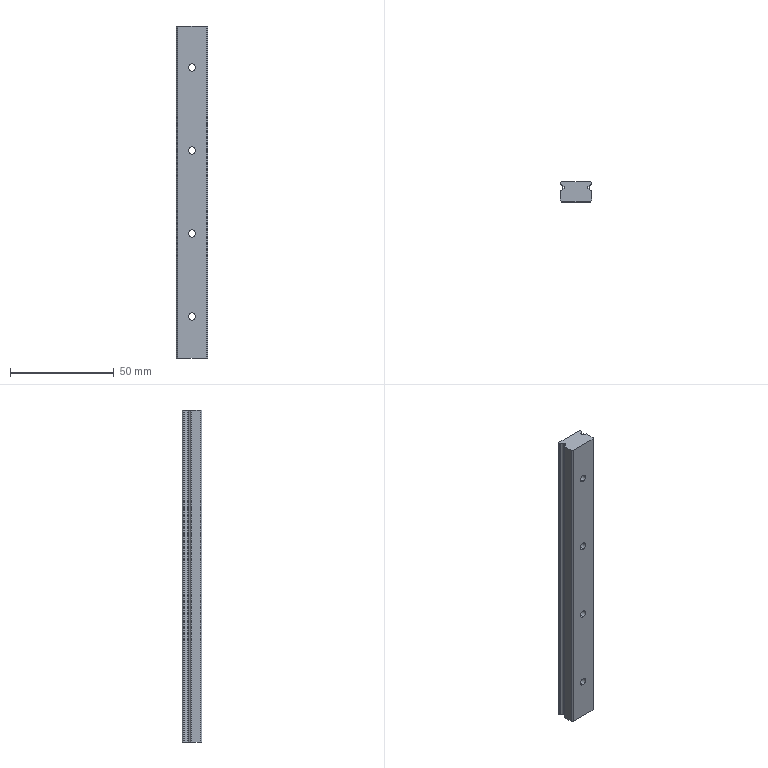Part | NX | features BREP 1 | 1 solid | 47 faces | box 15 x 9.5 x 160 mm | volume 20810 mm3 | cylinder 27 | plane 20 | commonest cylinder face diameters 3.5 x8 6 x8 0.4 x4 3.43 x4 0.8 x3
STEP:
#1=CARTESIAN_POINT('',(0.,-11.,-143.));
#2=VERTEX_POINT('',#1);
#3=CARTESIAN_POINT('',(0.,-11.,-137.));
#4=VERTEX_POINT('',#3);
#5=CARTESIAN_POINT('',(0.,-11.,-140.));
#6=DIRECTION('',(0.,1.,0.));
#7=DIRECTION('',(0.,0.,1.));
#8=AXIS2_PLACEMENT_3D('',#5,#6,#7);
#9=CIRCLE('',#8,3.);
#10=EDGE_CURVE('',#2,#4,#9,.T.);
#11=ORIENTED_EDGE('',*,*,#10,.F.);
#12=CARTESIAN_POINT('',(0.,-6.5,-143.));
#13=VERTEX_POINT('',#12);
#14=CARTESIAN_POINT('',(0.,-6.5,-143.));
#15=DIRECTION('',(0.,1.,0.));
#16=VECTOR('',#15,1000.);
#17=LINE('',#14,#16);
#18=EDGE_CURVE('',#2,#13,#17,.T.);
#19=ORIENTED_EDGE('',*,*,#18,.T.);
#20=CARTESIAN_POINT('',(0.,-6.5,-137.));
#21=VERTEX_POINT('',#20);
#22=CARTESIAN_POINT('',(0.,-6.5,-140.));
#23=DIRECTION('',(0.,1.,0.));
#24=DIRECTION('',(0.,0.,1.));
#25=AXIS2_PLACEMENT_3D('',#22,#23,#24);
#26=CIRCLE('',#25,3.);
#27=EDGE_CURVE('',#13,#21,#26,.T.);
#28=ORIENTED_EDGE('',*,*,#27,.T.);
#29=CARTESIAN_POINT('',(0.,-6.5,-137.));
#30=DIRECTION('',(0.,1.,0.));
#31=VECTOR('',#30,1000.);
#32=LINE('',#29,#31);
#33=EDGE_CURVE('',#4,#21,#32,.T.);
#34=ORIENTED_EDGE('',*,*,#33,.F.);
#35=EDGE_LOOP('',(#11,#19,#28,#34));
#36=FACE_BOUND('',#35,.T.);
#37=CARTESIAN_POINT('',(0.,-6.5,-140.));
#38=DIRECTION('',(0.,1.,0.));
#39=DIRECTION('',(0.,0.,-1.));
#40=AXIS2_PLACEMENT_3D('',#37,#38,#39);
#41=CYLINDRICAL_SURFACE('',#40,3.);
#42=ADVANCED_FACE('',(#36),#41,.F.);
#43=CARTESIAN_POINT('',(0.,-16.,-141.75));
#44=VERTEX_POINT('',#43);
#45=CARTESIAN_POINT('',(0.,-16.,-138.25));
#46=VERTEX_POINT('',#45);
#47=CARTESIAN_POINT('',(0.,-16.,-140.));
#48=DIRECTION('',(0.,1.,0.));
#49=DIRECTION('',(0.,0.,1.));
#50=AXIS2_PLACEMENT_3D('',#47,#48,#49);
#51=CIRCLE('',#50,1.75);
#52=EDGE_CURVE('',#44,#46,#51,.T.);
#53=ORIENTED_EDGE('',*,*,#52,.F.);
#54=CARTESIAN_POINT('',(0.,-11.,-141.75));
#55=VERTEX_POINT('',#54);
#56=CARTESIAN_POINT('',(0.,-6.5,-141.75));
#57=DIRECTION('',(0.,1.,0.));
#58=VECTOR('',#57,1000.);
#59=LINE('',#56,#58);
#60=EDGE_CURVE('',#44,#55,#59,.T.);
#61=ORIENTED_EDGE('',*,*,#60,.T.);
#62=CARTESIAN_POINT('',(0.,-11.,-138.25));
#63=VERTEX_POINT('',#62);
#64=CARTESIAN_POINT('',(0.,-11.,-140.));
#65=DIRECTION('',(0.,1.,0.));
#66=DIRECTION('',(0.,0.,1.));
#67=AXIS2_PLACEMENT_3D('',#64,#65,#66);
#68=CIRCLE('',#67,1.75);
#69=EDGE_CURVE('',#55,#63,#68,.T.);
#70=ORIENTED_EDGE('',*,*,#69,.T.);
#71=CARTESIAN_POINT('',(0.,-6.5,-138.25));
#72=DIRECTION('',(0.,1.,0.));
#73=VECTOR('',#72,1000.);
#74=LINE('',#71,#73);
#75=EDGE_CURVE('',#46,#63,#74,.T.);
#76=ORIENTED_EDGE('',*,*,#75,.F.);
#77=EDGE_LOOP('',(#53,#61,#70,#76));
#78=FACE_BOUND('',#77,.T.);
#79=CARTESIAN_POINT('',(0.,-6.5,-140.));
#80=DIRECTION('',(0.,1.,0.));
#81=DIRECTION('',(0.,0.,-1.));
#82=AXIS2_PLACEMENT_3D('',#79,#80,#81);
#83=CYLINDRICAL_SURFACE('',#82,1.75);
#84=ADVANCED_FACE('',(#78),#83,.F.);
#85=CARTESIAN_POINT('',(0.,-11.,-103.));
#86=VERTEX_POINT('',#85);
#87=CARTESIAN_POINT('',(0.,-11.,-97.));
#88=VERTEX_POINT('',#87);
#89=CARTESIAN_POINT('',(0.,-11.,-100.));
#90=DIRECTION('',(0.,1.,0.));
#91=DIRECTION('',(0.,0.,1.));
#92=AXIS2_PLACEMENT_3D('',#89,#90,#91);
#93=CIRCLE('',#92,3.);
#94=EDGE_CURVE('',#86,#88,#93,.T.);
#95=ORIENTED_EDGE('',*,*,#94,.F.);
#96=CARTESIAN_POINT('',(0.,-6.5,-103.));
#97=VERTEX_POINT('',#96);
#98=CARTESIAN_POINT('',(0.,-6.5,-103.));
#99=DIRECTION('',(0.,1.,0.));
#100=VECTOR('',#99,1000.);
#101=LINE('',#98,#100);
#102=EDGE_CURVE('',#86,#97,#101,.T.);
#103=ORIENTED_EDGE('',*,*,#102,.T.);
#104=CARTESIAN_POINT('',(0.,-6.5,-97.));
#105=VERTEX_POINT('',#104);
#106=CARTESIAN_POINT('',(0.,-6.5,-100.));
#107=DIRECTION('',(0.,1.,0.));
#108=DIRECTION('',(0.,0.,1.));
#109=AXIS2_PLACEMENT_3D('',#106,#107,#108);
#110=CIRCLE('',#109,3.);
#111=EDGE_CURVE('',#97,#105,#110,.T.);
#112=ORIENTED_EDGE('',*,*,#111,.T.);
#113=CARTESIAN_POINT('',(0.,-6.5,-97.));
#114=DIRECTION('',(0.,1.,0.));
#115=VECTOR('',#114,1000.);
#116=LINE('',#113,#115);
#117=EDGE_CURVE('',#88,#105,#116,.T.);
#118=ORIENTED_EDGE('',*,*,#117,.F.);
#119=EDGE_LOOP('',(#95,#103,#112,#118));
#120=FACE_BOUND('',#119,.T.);
#121=CARTESIAN_POINT('',(0.,-6.5,-100.));
#122=DIRECTION('',(0.,1.,0.));
#123=DIRECTION('',(0.,0.,-1.));
#124=AXIS2_PLACEMENT_3D('',#121,#122,#123);
#125=CYLINDRICAL_SURFACE('',#124,3.);
#126=ADVANCED_FACE('',(#120),#125,.F.);
#127=CARTESIAN_POINT('',(0.,-16.,-101.75));
#128=VERTEX_POINT('',#127);
#129=CARTESIAN_POINT('',(0.,-16.,-98.25));
#130=VERTEX_POINT('',#129);
#131=CARTESIAN_POINT('',(0.,-16.,-100.));
#132=DIRECTION('',(0.,1.,0.));
#133=DIRECTION('',(0.,0.,1.));
#134=AXIS2_PLACEMENT_3D('',#131,#132,#133);
#135=CIRCLE('',#134,1.75);
#136=EDGE_CURVE('',#128,#130,#135,.T.);
#137=ORIENTED_EDGE('',*,*,#136,.F.);
#138=CARTESIAN_POINT('',(0.,-11.,-101.75));
#139=VERTEX_POINT('',#138);
#140=CARTESIAN_POINT('',(0.,-6.5,-101.75));
#141=DIRECTION('',(0.,1.,0.));
#142=VECTOR('',#141,1000.);
#143=LINE('',#140,#142);
#144=EDGE_CURVE('',#128,#139,#143,.T.);
#145=ORIENTED_EDGE('',*,*,#144,.T.);
#146=CARTESIAN_POINT('',(0.,-11.,-98.25));
#147=VERTEX_POINT('',#146);
#148=CARTESIAN_POINT('',(0.,-11.,-100.));
#149=DIRECTION('',(0.,1.,0.));
#150=DIRECTION('',(0.,0.,1.));
#151=AXIS2_PLACEMENT_3D('',#148,#149,#150);
#152=CIRCLE('',#151,1.75);
#153=EDGE_CURVE('',#139,#147,#152,.T.);
#154=ORIENTED_EDGE('',*,*,#153,.T.);
#155=CARTESIAN_POINT('',(0.,-6.5,-98.25));
#156=DIRECTION('',(0.,1.,0.));
#157=VECTOR('',#156,1000.);
#158=LINE('',#155,#157);
#159=EDGE_CURVE('',#130,#147,#158,.T.);
#160=ORIENTED_EDGE('',*,*,#159,.F.);
#161=EDGE_LOOP('',(#137,#145,#154,#160));
#162=FACE_BOUND('',#161,.T.);
#163=CARTESIAN_POINT('',(0.,-6.5,-100.));
#164=DIRECTION('',(0.,1.,0.));
#165=DIRECTION('',(0.,0.,-1.));
#166=AXIS2_PLACEMENT_3D('',#163,#164,#165);
#167=CYLINDRICAL_SURFACE('',#166,1.75);
#168=ADVANCED_FACE('',(#162),#167,.F.);
#169=CARTESIAN_POINT('',(0.,-11.,-63.));
#170=VERTEX_POINT('',#169);
#171=CARTESIAN_POINT('',(0.,-11.,-57.));
#172=VERTEX_POINT('',#171);
#173=CARTESIAN_POINT('',(0.,-11.,-60.));
#174=DIRECTION('',(0.,1.,0.));
#175=DIRECTION('',(0.,0.,1.));
#176=AXIS2_PLACEMENT_3D('',#173,#174,#175);
#177=CIRCLE('',#176,3.);
#178=EDGE_CURVE('',#170,#172,#177,.T.);
#179=ORIENTED_EDGE('',*,*,#178,.F.);
#180=CARTESIAN_POINT('',(0.,-6.5,-63.));
#181=VERTEX_POINT('',#180);
#182=CARTESIAN_POINT('',(0.,-6.5,-63.));
#183=DIRECTION('',(0.,1.,0.));
#184=VECTOR('',#183,1000.);
#185=LINE('',#182,#184);
#186=EDGE_CURVE('',#170,#181,#185,.T.);
#187=ORIENTED_EDGE('',*,*,#186,.T.);
#188=CARTESIAN_POINT('',(0.,-6.5,-57.));
#189=VERTEX_POINT('',#188);
#190=CARTESIAN_POINT('',(0.,-6.5,-60.));
#191=DIRECTION('',(0.,1.,0.));
#192=DIRECTION('',(0.,0.,1.));
#193=AXIS2_PLACEMENT_3D('',#190,#191,#192);
#194=CIRCLE('',#193,3.);
#195=EDGE_CURVE('',#181,#189,#194,.T.);
#196=ORIENTED_EDGE('',*,*,#195,.T.);
#197=CARTESIAN_POINT('',(0.,-6.5,-57.));
#198=DIRECTION('',(0.,1.,0.));
#199=VECTOR('',#198,1000.);
#200=LINE('',#197,#199);
#201=EDGE_CURVE('',#172,#189,#200,.T.);
#202=ORIENTED_EDGE('',*,*,#201,.F.);
#203=EDGE_LOOP('',(#179,#187,#196,#202));
#204=FACE_BOUND('',#203,.T.);
#205=CARTESIAN_POINT('',(0.,-6.5,-60.));
#206=DIRECTION('',(0.,1.,0.));
#207=DIRECTION('',(0.,0.,-1.));
#208=AXIS2_PLACEMENT_3D('',#205,#206,#207);
#209=CYLINDRICAL_SURFACE('',#208,3.);
#210=ADVANCED_FACE('',(#204),#209,.F.);
#211=CARTESIAN_POINT('',(0.,-16.,-61.75));
#212=VERTEX_POINT('',#211);
#213=CARTESIAN_POINT('',(0.,-16.,-58.25));
#214=VERTEX_POINT('',#213);
#215=CARTESIAN_POINT('',(0.,-16.,-60.));
#216=DIRECTION('',(0.,1.,0.));
#217=DIRECTION('',(0.,0.,1.));
#218=AXIS2_PLACEMENT_3D('',#215,#216,#217);
#219=CIRCLE('',#218,1.75);
#220=EDGE_CURVE('',#212,#214,#219,.T.);
#221=ORIENTED_EDGE('',*,*,#220,.F.);
#222=CARTESIAN_POINT('',(0.,-11.,-61.75));
#223=VERTEX_POINT('',#222);
#224=CARTESIAN_POINT('',(0.,-6.5,-61.75));
#225=DIRECTION('',(0.,1.,0.));
#226=VECTOR('',#225,1000.);
#227=LINE('',#224,#226);
#228=EDGE_CURVE('',#212,#223,#227,.T.);
#229=ORIENTED_EDGE('',*,*,#228,.T.);
#230=CARTESIAN_POINT('',(0.,-11.,-58.25));
#231=VERTEX_POINT('',#230);
#232=CARTESIAN_POINT('',(0.,-11.,-60.));
#233=DIRECTION('',(0.,1.,0.));
#234=DIRECTION('',(0.,0.,1.));
#235=AXIS2_PLACEMENT_3D('',#232,#233,#234);
#236=CIRCLE('',#235,1.75);
#237=EDGE_CURVE('',#223,#231,#236,.T.);
#238=ORIENTED_EDGE('',*,*,#237,.T.);
#239=CARTESIAN_POINT('',(0.,-6.5,-58.25));
#240=DIRECTION('',(0.,1.,0.));
#241=VECTOR('',#240,1000.);
#242=LINE('',#239,#241);
#243=EDGE_CURVE('',#214,#231,#242,.T.);
#244=ORIENTED_EDGE('',*,*,#243,.F.);
#245=EDGE_LOOP('',(#221,#229,#238,#244));
#246=FACE_BOUND('',#245,.T.);
#247=CARTESIAN_POINT('',(0.,-6.5,-60.));
#248=DIRECTION('',(0.,1.,0.));
#249=DIRECTION('',(0.,0.,-1.));
#250=AXIS2_PLACEMENT_3D('',#247,#248,#249);
#251=CYLINDRICAL_SURFACE('',#250,1.75);
#252=ADVANCED_FACE('',(#246),#251,.F.);
#253=CARTESIAN_POINT('',(0.,-11.,-23.));
#254=VERTEX_POINT('',#253);
#255=CARTESIAN_POINT('',(0.,-11.,-17.));
#256=VERTEX_POINT('',#255);
#257=CARTESIAN_POINT('',(0.,-11.,-20.));
#258=DIRECTION('',(0.,1.,0.));
#259=DIRECTION('',(0.,0.,1.));
#260=AXIS2_PLACEMENT_3D('',#257,#258,#259);
#261=CIRCLE('',#260,3.);
#262=EDGE_CURVE('',#254,#256,#261,.T.);
#263=ORIENTED_EDGE('',*,*,#262,.F.);
#264=CARTESIAN_POINT('',(0.,-6.5,-23.));
#265=VERTEX_POINT('',#264);
#266=CARTESIAN_POINT('',(0.,-6.5,-23.));
#267=DIRECTION('',(0.,1.,0.));
#268=VECTOR('',#267,1000.);
#269=LINE('',#266,#268);
#270=EDGE_CURVE('',#254,#265,#269,.T.);
#271=ORIENTED_EDGE('',*,*,#270,.T.);
#272=CARTESIAN_POINT('',(0.,-6.5,-17.));
#273=VERTEX_POINT('',#272);
#274=CARTESIAN_POINT('',(0.,-6.5,-20.));
#275=DIRECTION('',(0.,1.,0.));
#276=DIRECTION('',(0.,0.,1.));
#277=AXIS2_PLACEMENT_3D('',#274,#275,#276);
#278=CIRCLE('',#277,3.);
#279=EDGE_CURVE('',#265,#273,#278,.T.);
#280=ORIENTED_EDGE('',*,*,#279,.T.);
#281=CARTESIAN_POINT('',(0.,-6.5,-17.));
#282=DIRECTION('',(0.,1.,0.));
#283=VECTOR('',#282,1000.);
#284=LINE('',#281,#283);
#285=EDGE_CURVE('',#256,#273,#284,.T.);
#286=ORIENTED_EDGE('',*,*,#285,.F.);
#287=EDGE_LOOP('',(#263,#271,#280,#286));
#288=FACE_BOUND('',#287,.T.);
#289=CARTESIAN_POINT('',(0.,-6.5,-20.));
#290=DIRECTION('',(0.,1.,0.));
#291=DIRECTION('',(0.,0.,-1.));
#292=AXIS2_PLACEMENT_3D('',#289,#290,#291);
#293=CYLINDRICAL_SURFACE('',#292,3.);
#294=ADVANCED_FACE('',(#288),#293,.F.);
#295=CARTESIAN_POINT('',(0.,-16.,-21.75));
#296=VERTEX_POINT('',#295);
#297=CARTESIAN_POINT('',(0.,-16.,-18.25));
#298=VERTEX_POINT('',#297);
#299=CARTESIAN_POINT('',(0.,-16.,-20.));
#300=DIRECTION('',(0.,1.,0.));
#301=DIRECTION('',(0.,0.,1.));
#302=AXIS2_PLACEMENT_3D('',#299,#300,#301);
#303=CIRCLE('',#302,1.75);
#304=EDGE_CURVE('',#296,#298,#303,.T.);
#305=ORIENTED_EDGE('',*,*,#304,.F.);
#306=CARTESIAN_POINT('',(0.,-11.,-21.75));
#307=VERTEX_POINT('',#306);
#308=CARTESIAN_POINT('',(0.,-6.5,-21.75));
#309=DIRECTION('',(0.,1.,0.));
#310=VECTOR('',#309,1000.);
#311=LINE('',#308,#310);
#312=EDGE_CURVE('',#296,#307,#311,.T.);
#313=ORIENTED_EDGE('',*,*,#312,.T.);
#314=CARTESIAN_POINT('',(0.,-11.,-18.25));
#315=VERTEX_POINT('',#314);
#316=CARTESIAN_POINT('',(0.,-11.,-20.));
#317=DIRECTION('',(0.,1.,0.));
#318=DIRECTION('',(0.,0.,1.));
#319=AXIS2_PLACEMENT_3D('',#316,#317,#318);
#320=CIRCLE('',#319,1.75);
#321=EDGE_CURVE('',#307,#315,#320,.T.);
#322=ORIENTED_EDGE('',*,*,#321,.T.);
#323=CARTESIAN_POINT('',(0.,-6.5,-18.25));
#324=DIRECTION('',(0.,1.,0.));
#325=VECTOR('',#324,1000.);
#326=LINE('',#323,#325);
#327=EDGE_CURVE('',#298,#315,#326,.T.);
#328=ORIENTED_EDGE('',*,*,#327,.F.);
#329=EDGE_LOOP('',(#305,#313,#322,#328));
#330=FACE_BOUND('',#329,.T.);
#331=CARTESIAN_POINT('',(0.,-6.5,-20.));
#332=DIRECTION('',(0.,1.,0.));
#333=DIRECTION('',(0.,0.,-1.));
#334=AXIS2_PLACEMENT_3D('',#331,#332,#333);
#335=CYLINDRICAL_SURFACE('',#334,1.75);
#336=ADVANCED_FACE('',(#330),#335,.F.);
#337=CARTESIAN_POINT('',(-5.767,-8.859,-160.));
#338=VERTEX_POINT('',#337);
#339=CARTESIAN_POINT('',(-5.45,-9.25,-160.));
#340=VERTEX_POINT('',#339);
#341=CARTESIAN_POINT('',(-5.85,-9.25,-160.));
#342=DIRECTION('',(0.,0.,-1.));
#343=DIRECTION('',(-1.,0.,0.));
#344=AXIS2_PLACEMENT_3D('',#341,#342,#343);
#345=CIRCLE('',#344,0.4);
#346=EDGE_CURVE('',#338,#340,#345,.T.);
#347=ORIENTED_EDGE('',*,*,#346,.T.);
#348=CARTESIAN_POINT('',(-5.45,-9.25,0.));
#349=VERTEX_POINT('',#348);
#350=CARTESIAN_POINT('',(-5.45,-9.25,-160.));
#351=DIRECTION('',(0.,0.,1.));
#352=VECTOR('',#351,1000.);
#353=LINE('',#350,#352);
#354=EDGE_CURVE('',#340,#349,#353,.T.);
#355=ORIENTED_EDGE('',*,*,#354,.T.);
#356=CARTESIAN_POINT('',(-5.767,-8.859,0.));
#357=VERTEX_POINT('',#356);
#358=CARTESIAN_POINT('',(-5.85,-9.25,0.));
#359=DIRECTION('',(0.,0.,-1.));
#360=DIRECTION('',(-1.,0.,0.));
#361=AXIS2_PLACEMENT_3D('',#358,#359,#360);
#362=CIRCLE('',#361,0.4);
#363=EDGE_CURVE('',#357,#349,#362,.T.);
#364=ORIENTED_EDGE('',*,*,#363,.F.);
#365=CARTESIAN_POINT('',(-5.767,-8.859,-160.));
#366=DIRECTION('',(0.,0.,1.));
#367=VECTOR('',#366,1000.);
#368=LINE('',#365,#367);
#369=EDGE_CURVE('',#338,#357,#368,.T.);
#370=ORIENTED_EDGE('',*,*,#369,.F.);
#371=EDGE_LOOP('',(#347,#355,#364,#370));
#372=FACE_BOUND('',#371,.T.);
#373=CARTESIAN_POINT('',(-5.85,-9.25,-160.));
#374=DIRECTION('',(0.,0.,1.));
#375=DIRECTION('',(-1.,0.,0.));
#376=AXIS2_PLACEMENT_3D('',#373,#374,#375);
#377=CYLINDRICAL_SURFACE('',#376,0.4);
#378=ADVANCED_FACE('',(#372),#377,.F.);
#379=CARTESIAN_POINT('',(-7.362,-10.791,0.));
#380=VERTEX_POINT('',#379);
#381=CARTESIAN_POINT('',(-7.5,-10.982,0.));
#382=VERTEX_POINT('',#381);
#383=CARTESIAN_POINT('',(-7.3,-10.982,0.));
#384=DIRECTION('',(0.,0.,1.));
#385=DIRECTION('',(1.,0.,0.));
#386=AXIS2_PLACEMENT_3D('',#383,#384,#385);
#387=CIRCLE('',#386,0.2);
#388=EDGE_CURVE('',#380,#382,#387,.T.);
#389=ORIENTED_EDGE('',*,*,#388,.F.);
#390=CARTESIAN_POINT('',(-7.362,-10.791,-160.));
#391=VERTEX_POINT('',#390);
#392=CARTESIAN_POINT('',(-7.362,-10.791,-160.));
#393=DIRECTION('',(0.,0.,1.));
#394=VECTOR('',#393,1000.);
#395=LINE('',#392,#394);
#396=EDGE_CURVE('',#391,#380,#395,.T.);
#397=ORIENTED_EDGE('',*,*,#396,.F.);
#398=CARTESIAN_POINT('',(-7.5,-10.982,-160.));
#399=VERTEX_POINT('',#398);
#400=CARTESIAN_POINT('',(-7.3,-10.982,-160.));
#401=DIRECTION('',(0.,0.,1.));
#402=DIRECTION('',(1.,0.,0.));
#403=AXIS2_PLACEMENT_3D('',#400,#401,#402);
#404=CIRCLE('',#403,0.2);
#405=EDGE_CURVE('',#391,#399,#404,.T.);
#406=ORIENTED_EDGE('',*,*,#405,.T.);
#407=CARTESIAN_POINT('',(-7.5,-10.982,-160.));
#408=DIRECTION('',(0.,0.,1.));
#409=VECTOR('',#408,1000.);
#410=LINE('',#407,#409);
#411=EDGE_CURVE('',#399,#382,#410,.T.);
#412=ORIENTED_EDGE('',*,*,#411,.T.);
#413=EDGE_LOOP('',(#389,#397,#406,#412));
#414=FACE_BOUND('',#413,.T.);
#415=CARTESIAN_POINT('',(-7.3,-10.982,-160.));
#416=DIRECTION('',(0.,0.,1.));
#417=DIRECTION('',(-1.,0.,0.));
#418=AXIS2_PLACEMENT_3D('',#415,#416,#417);
#419=CYLINDRICAL_SURFACE('',#418,0.2);
#420=ADVANCED_FACE('',(#414),#419,.T.);
#421=CARTESIAN_POINT('',(-6.28,-9.75,0.));
#422=VERTEX_POINT('',#421);
#423=CARTESIAN_POINT('',(-7.89,-9.16,0.));
#424=DIRECTION('',(0.,0.,-1.));
#425=DIRECTION('',(-1.,0.,0.));
#426=AXIS2_PLACEMENT_3D('',#423,#424,#425);
#427=CIRCLE('',#426,1.715);
#428=EDGE_CURVE('',#422,#380,#427,.T.);
#429=ORIENTED_EDGE('',*,*,#428,.F.);
#430=CARTESIAN_POINT('',(-6.28,-9.75,-160.));
#431=VERTEX_POINT('',#430);
#432=CARTESIAN_POINT('',(-6.28,-9.75,-160.));
#433=DIRECTION('',(0.,0.,1.));
#434=VECTOR('',#433,1000.);
#435=LINE('',#432,#434);
#436=EDGE_CURVE('',#431,#422,#435,.T.);
#437=ORIENTED_EDGE('',*,*,#436,.F.);
#438=CARTESIAN_POINT('',(-7.89,-9.16,-160.));
#439=DIRECTION('',(0.,0.,-1.));
#440=DIRECTION('',(-1.,0.,0.));
#441=AXIS2_PLACEMENT_3D('',#438,#439,#440);
#442=CIRCLE('',#441,1.715);
#443=EDGE_CURVE('',#431,#391,#442,.T.);
#444=ORIENTED_EDGE('',*,*,#443,.T.);
#445=ORIENTED_EDGE('',*,*,#396,.T.);
#446=EDGE_LOOP('',(#429,#437,#444,#445));
#447=FACE_BOUND('',#446,.T.);
#448=CARTESIAN_POINT('',(-7.89,-9.16,-160.));
#449=DIRECTION('',(0.,0.,1.));
#450=DIRECTION('',(-1.,0.,0.));
#451=AXIS2_PLACEMENT_3D('',#448,#449,#450);
#452=CYLINDRICAL_SURFACE('',#451,1.715);
#453=ADVANCED_FACE('',(#447),#452,.F.);
#454=CARTESIAN_POINT('',(-5.767,-9.641,0.));
#455=VERTEX_POINT('',#454);
#456=CARTESIAN_POINT('',(-5.767,-9.641,0.));
#457=DIRECTION('',(-0.9781,-0.2079,0.));
#458=VECTOR('',#457,1000.);
#459=LINE('',#456,#458);
#460=EDGE_CURVE('',#455,#422,#459,.T.);
#461=ORIENTED_EDGE('',*,*,#460,.F.);
#462=CARTESIAN_POINT('',(-5.767,-9.641,-160.));
#463=VERTEX_POINT('',#462);
#464=CARTESIAN_POINT('',(-5.767,-9.641,-160.));
#465=DIRECTION('',(0.,0.,1.));
#466=VECTOR('',#465,1000.);
#467=LINE('',#464,#466);
#468=EDGE_CURVE('',#463,#455,#467,.T.);
#469=ORIENTED_EDGE('',*,*,#468,.F.);
#470=CARTESIAN_POINT('',(-5.767,-9.641,-160.));
#471=DIRECTION('',(-0.9781,-0.2079,0.));
#472=VECTOR('',#471,1000.);
#473=LINE('',#470,#472);
#474=EDGE_CURVE('',#463,#431,#473,.T.);
#475=ORIENTED_EDGE('',*,*,#474,.T.);
#476=ORIENTED_EDGE('',*,*,#436,.T.);
#477=EDGE_LOOP('',(#461,#469,#475,#476));
#478=FACE_BOUND('',#477,.T.);
#479=CARTESIAN_POINT('',(-5.767,-9.641,-160.));
#480=DIRECTION('',(-0.2079,0.9781,0.));
#481=DIRECTION('',(0.9781,0.2079,0.));
#482=AXIS2_PLACEMENT_3D('',#479,#480,#481);
#483=PLANE('',#482);
#484=ADVANCED_FACE('',(#478),#483,.T.);
#485=ORIENTED_EDGE('',*,*,#354,.F.);
#486=CARTESIAN_POINT('',(-5.85,-9.25,-160.));
#487=DIRECTION('',(0.,0.,-1.));
#488=DIRECTION('',(-1.,0.,0.));
#489=AXIS2_PLACEMENT_3D('',#486,#487,#488);
#490=CIRCLE('',#489,0.4);
#491=EDGE_CURVE('',#340,#463,#490,.T.);
#492=ORIENTED_EDGE('',*,*,#491,.T.);
#493=ORIENTED_EDGE('',*,*,#468,.T.);
#494=CARTESIAN_POINT('',(-5.85,-9.25,0.));
#495=DIRECTION('',(0.,0.,-1.));
#496=DIRECTION('',(-1.,0.,0.));
#497=AXIS2_PLACEMENT_3D('',#494,#495,#496);
#498=CIRCLE('',#497,0.4);
#499=EDGE_CURVE('',#349,#455,#498,.T.);
#500=ORIENTED_EDGE('',*,*,#499,.F.);
#501=EDGE_LOOP('',(#485,#492,#493,#500));
#502=FACE_BOUND('',#501,.T.);
#503=CARTESIAN_POINT('',(-5.85,-9.25,-160.));
#504=DIRECTION('',(0.,0.,1.));
#505=DIRECTION('',(-1.,0.,0.));
#506=AXIS2_PLACEMENT_3D('',#503,#504,#505);
#507=CYLINDRICAL_SURFACE('',#506,0.4);
#508=ADVANCED_FACE('',(#502),#507,.F.);
#509=CARTESIAN_POINT('',(-6.28,-8.75,0.));
#510=VERTEX_POINT('',#509);
#511=CARTESIAN_POINT('',(-6.28,-8.75,0.));
#512=DIRECTION('',(0.9781,-0.2079,0.));
#513=VECTOR('',#512,1000.);
#514=LINE('',#511,#513);
#515=EDGE_CURVE('',#510,#357,#514,.T.);
#516=ORIENTED_EDGE('',*,*,#515,.F.);
#517=CARTESIAN_POINT('',(-6.28,-8.75,-160.));
#518=VERTEX_POINT('',#517);
#519=CARTESIAN_POINT('',(-6.28,-8.75,-160.));
#520=DIRECTION('',(0.,0.,1.));
#521=VECTOR('',#520,1000.);
#522=LINE('',#519,#521);
#523=EDGE_CURVE('',#518,#510,#522,.T.);
#524=ORIENTED_EDGE('',*,*,#523,.F.);
#525=CARTESIAN_POINT('',(-6.28,-8.75,-160.));
#526=DIRECTION('',(0.9781,-0.2079,0.));
#527=VECTOR('',#526,1000.);
#528=LINE('',#525,#527);
#529=EDGE_CURVE('',#518,#338,#528,.T.);
#530=ORIENTED_EDGE('',*,*,#529,.T.);
#531=ORIENTED_EDGE('',*,*,#369,.T.);
#532=EDGE_LOOP('',(#516,#524,#530,#531));
#533=FACE_BOUND('',#532,.T.);
#534=CARTESIAN_POINT('',(-6.28,-8.75,-160.));
#535=DIRECTION('',(-0.2079,-0.9781,0.));
#536=DIRECTION('',(-0.9781,0.2079,0.));
#537=AXIS2_PLACEMENT_3D('',#534,#535,#536);
#538=PLANE('',#537);
#539=ADVANCED_FACE('',(#533),#538,.T.);
#540=CARTESIAN_POINT('',(-7.35,-7.712,0.));
#541=VERTEX_POINT('',#540);
#542=CARTESIAN_POINT('',(-7.89,-9.34,0.));
#543=DIRECTION('',(0.,0.,-1.));
#544=DIRECTION('',(-1.,0.,0.));
#545=AXIS2_PLACEMENT_3D('',#542,#543,#544);
#546=CIRCLE('',#545,1.715);
#547=EDGE_CURVE('',#541,#510,#546,.T.);
#548=ORIENTED_EDGE('',*,*,#547,.F.);
#549=CARTESIAN_POINT('',(-7.35,-7.712,-160.));
#550=VERTEX_POINT('',#549);
#551=CARTESIAN_POINT('',(-7.35,-7.712,-160.));
#552=DIRECTION('',(0.,0.,1.));
#553=VECTOR('',#552,1000.);
#554=LINE('',#551,#553);
#555=EDGE_CURVE('',#550,#541,#554,.T.);
#556=ORIENTED_EDGE('',*,*,#555,.F.);
#557=CARTESIAN_POINT('',(-7.89,-9.34,-160.));
#558=DIRECTION('',(0.,0.,-1.));
#559=DIRECTION('',(-1.,0.,0.));
#560=AXIS2_PLACEMENT_3D('',#557,#558,#559);
#561=CIRCLE('',#560,1.715);
#562=EDGE_CURVE('',#550,#518,#561,.T.);
#563=ORIENTED_EDGE('',*,*,#562,.T.);
#564=ORIENTED_EDGE('',*,*,#523,.T.);
#565=EDGE_LOOP('',(#548,#556,#563,#564));
#566=FACE_BOUND('',#565,.T.);
#567=CARTESIAN_POINT('',(-7.89,-9.34,-160.));
#568=DIRECTION('',(0.,0.,1.));
#569=DIRECTION('',(-1.,0.,0.));
#570=AXIS2_PLACEMENT_3D('',#567,#568,#569);
#571=CYLINDRICAL_SURFACE('',#570,1.715);
#572=ADVANCED_FACE('',(#566),#571,.F.);
#573=CARTESIAN_POINT('',(-7.488,-7.522,0.));
#574=VERTEX_POINT('',#573);
#575=CARTESIAN_POINT('',(-7.287,-7.522,0.));
#576=DIRECTION('',(0.,0.,1.));
#577=DIRECTION('',(1.,0.,0.));
#578=AXIS2_PLACEMENT_3D('',#575,#576,#577);
#579=CIRCLE('',#578,0.2);
#580=EDGE_CURVE('',#574,#541,#579,.T.);
#581=ORIENTED_EDGE('',*,*,#580,.F.);
#582=CARTESIAN_POINT('',(-7.488,-7.522,-160.));
#583=VERTEX_POINT('',#582);
#584=CARTESIAN_POINT('',(-7.488,-7.522,-160.));
#585=DIRECTION('',(0.,0.,1.));
#586=VECTOR('',#585,1000.);
#587=LINE('',#584,#586);
#588=EDGE_CURVE('',#583,#574,#587,.T.);
#589=ORIENTED_EDGE('',*,*,#588,.F.);
#590=CARTESIAN_POINT('',(-7.287,-7.522,-160.));
#591=DIRECTION('',(0.,0.,1.));
#592=DIRECTION('',(1.,0.,0.));
#593=AXIS2_PLACEMENT_3D('',#590,#591,#592);
#594=CIRCLE('',#593,0.2);
#595=EDGE_CURVE('',#583,#550,#594,.T.);
#596=ORIENTED_EDGE('',*,*,#595,.T.);
#597=ORIENTED_EDGE('',*,*,#555,.T.);
#598=EDGE_LOOP('',(#581,#589,#596,#597));
#599=FACE_BOUND('',#598,.T.);
#600=CARTESIAN_POINT('',(-7.287,-7.522,-160.));
#601=DIRECTION('',(0.,0.,1.));
#602=DIRECTION('',(-1.,0.,0.));
#603=AXIS2_PLACEMENT_3D('',#600,#601,#602);
#604=CYLINDRICAL_SURFACE('',#603,0.2);
#605=ADVANCED_FACE('',(#599),#604,.T.);
#606=CARTESIAN_POINT('',(-7.488,-7.,0.));
#607=VERTEX_POINT('',#606);
#608=CARTESIAN_POINT('',(-7.488,-7.,0.));
#609=DIRECTION('',(0.,-1.,0.));
#610=VECTOR('',#609,1000.);
#611=LINE('',#608,#610);
#612=EDGE_CURVE('',#607,#574,#611,.T.);
#613=ORIENTED_EDGE('',*,*,#612,.F.);
#614=CARTESIAN_POINT('',(-7.488,-7.,-160.));
#615=VERTEX_POINT('',#614);
#616=CARTESIAN_POINT('',(-7.488,-7.,-160.));
#617=DIRECTION('',(0.,0.,1.));
#618=VECTOR('',#617,1000.);
#619=LINE('',#616,#618);
#620=EDGE_CURVE('',#615,#607,#619,.T.);
#621=ORIENTED_EDGE('',*,*,#620,.F.);
#622=CARTESIAN_POINT('',(-7.488,-7.,-160.));
#623=DIRECTION('',(0.,-1.,0.));
#624=VECTOR('',#623,1000.);
#625=LINE('',#622,#624);
#626=EDGE_CURVE('',#615,#583,#625,.T.);
#627=ORIENTED_EDGE('',*,*,#626,.T.);
#628=ORIENTED_EDGE('',*,*,#588,.T.);
#629=EDGE_LOOP('',(#613,#621,#627,#628));
#630=FACE_BOUND('',#629,.T.);
#631=CARTESIAN_POINT('',(-7.488,-7.,-160.));
#632=DIRECTION('',(-1.,0.,0.));
#633=DIRECTION('',(0.,0.,-1.));
#634=AXIS2_PLACEMENT_3D('',#631,#632,#633);
#635=PLANE('',#634);
#636=ADVANCED_FACE('',(#630),#635,.T.);
#637=CARTESIAN_POINT('',(-6.988,-6.5,0.));
#638=VERTEX_POINT('',#637);
#639=CARTESIAN_POINT('',(-6.988,-6.5,0.));
#640=DIRECTION('',(-0.7071,-0.7071,0.));
#641=VECTOR('',#640,1000.);
#642=LINE('',#639,#641);
#643=EDGE_CURVE('',#638,#607,#642,.T.);
#644=ORIENTED_EDGE('',*,*,#643,.F.);
#645=CARTESIAN_POINT('',(-6.988,-6.5,-160.));
#646=VERTEX_POINT('',#645);
#647=CARTESIAN_POINT('',(-6.988,-6.5,-160.));
#648=DIRECTION('',(0.,0.,1.));
#649=VECTOR('',#648,1000.);
#650=LINE('',#647,#649);
#651=EDGE_CURVE('',#646,#638,#650,.T.);
#652=ORIENTED_EDGE('',*,*,#651,.F.);
#653=CARTESIAN_POINT('',(-6.988,-6.5,-160.));
#654=DIRECTION('',(-0.7071,-0.7071,0.));
#655=VECTOR('',#654,1000.);
#656=LINE('',#653,#655);
#657=EDGE_CURVE('',#646,#615,#656,.T.);
#658=ORIENTED_EDGE('',*,*,#657,.T.);
#659=ORIENTED_EDGE('',*,*,#620,.T.);
#660=EDGE_LOOP('',(#644,#652,#658,#659));
#661=FACE_BOUND('',#660,.T.);
#662=CARTESIAN_POINT('',(-6.988,-6.5,-160.));
#663=DIRECTION('',(-0.7071,0.7071,0.));
#664=DIRECTION('',(0.7071,0.7071,0.));
#665=AXIS2_PLACEMENT_3D('',#662,#663,#664);
#666=PLANE('',#665);
#667=ADVANCED_FACE('',(#661),#666,.T.);
#668=CARTESIAN_POINT('',(0.,-6.5,-140.));
#669=DIRECTION('',(0.,1.,0.));
#670=DIRECTION('',(0.,0.,1.));
#671=AXIS2_PLACEMENT_3D('',#668,#669,#670);
#672=CIRCLE('',#671,3.);
#673=EDGE_CURVE('',#21,#13,#672,.T.);
#674=ORIENTED_EDGE('',*,*,#673,.F.);
#675=ORIENTED_EDGE('',*,*,#27,.F.);
#676=EDGE_LOOP('',(#674,#675));
#677=FACE_BOUND('',#676,.T.);
#678=CARTESIAN_POINT('',(0.,-6.5,-100.));
#679=DIRECTION('',(0.,1.,0.));
#680=DIRECTION('',(0.,0.,1.));
#681=AXIS2_PLACEMENT_3D('',#678,#679,#680);
#682=CIRCLE('',#681,3.);
#683=EDGE_CURVE('',#105,#97,#682,.T.);
#684=ORIENTED_EDGE('',*,*,#683,.F.);
#685=ORIENTED_EDGE('',*,*,#111,.F.);
#686=EDGE_LOOP('',(#684,#685));
#687=FACE_BOUND('',#686,.T.);
#688=CARTESIAN_POINT('',(0.,-6.5,-60.));
#689=DIRECTION('',(0.,1.,0.));
#690=DIRECTION('',(0.,0.,1.));
#691=AXIS2_PLACEMENT_3D('',#688,#689,#690);
#692=CIRCLE('',#691,3.);
#693=EDGE_CURVE('',#189,#181,#692,.T.);
#694=ORIENTED_EDGE('',*,*,#693,.F.);
#695=ORIENTED_EDGE('',*,*,#195,.F.);
#696=EDGE_LOOP('',(#694,#695));
#697=FACE_BOUND('',#696,.T.);
#698=CARTESIAN_POINT('',(0.,-6.5,-20.));
#699=DIRECTION('',(0.,1.,0.));
#700=DIRECTION('',(0.,0.,1.));
#701=AXIS2_PLACEMENT_3D('',#698,#699,#700);
#702=CIRCLE('',#701,3.);
#703=EDGE_CURVE('',#273,#265,#702,.T.);
#704=ORIENTED_EDGE('',*,*,#703,.F.);
#705=ORIENTED_EDGE('',*,*,#279,.F.);
#706=EDGE_LOOP('',(#704,#705));
#707=FACE_BOUND('',#706,.T.);
#708=CARTESIAN_POINT('',(6.987,-6.5,0.));
#709=VERTEX_POINT('',#708);
#710=CARTESIAN_POINT('',(6.987,-6.5,0.));
#711=DIRECTION('',(-1.,0.,0.));
#712=VECTOR('',#711,1000.);
#713=LINE('',#710,#712);
#714=EDGE_CURVE('',#709,#638,#713,.T.);
#715=ORIENTED_EDGE('',*,*,#714,.F.);
#716=CARTESIAN_POINT('',(6.987,-6.5,-160.));
#717=VERTEX_POINT('',#716);
#718=CARTESIAN_POINT('',(6.987,-6.5,-160.));
#719=DIRECTION('',(0.,0.,1.));
#720=VECTOR('',#719,1000.);
#721=LINE('',#718,#720);
#722=EDGE_CURVE('',#717,#709,#721,.T.);
#723=ORIENTED_EDGE('',*,*,#722,.F.);
#724=CARTESIAN_POINT('',(6.987,-6.5,-160.));
#725=DIRECTION('',(-1.,0.,0.));
#726=VECTOR('',#725,1000.);
#727=LINE('',#724,#726);
#728=EDGE_CURVE('',#717,#646,#727,.T.);
#729=ORIENTED_EDGE('',*,*,#728,.T.);
#730=ORIENTED_EDGE('',*,*,#651,.T.);
#731=EDGE_LOOP('',(#715,#723,#729,#730));
#732=FACE_BOUND('',#731,.T.);
#733=CARTESIAN_POINT('',(6.987,-6.5,-160.));
#734=DIRECTION('',(0.,1.,0.));
#735=DIRECTION('',(0.,0.,-1.));
#736=AXIS2_PLACEMENT_3D('',#733,#734,#735);
#737=PLANE('',#736);
#738=ADVANCED_FACE('',(#677,#687,#697,#707,#732),#737,.T.);
#739=CARTESIAN_POINT('',(7.487,-7.,0.));
#740=VERTEX_POINT('',#739);
#741=CARTESIAN_POINT('',(7.487,-7.,0.));
#742=DIRECTION('',(-0.7071,0.7071,0.));
#743=VECTOR('',#742,1000.);
#744=LINE('',#741,#743);
#745=EDGE_CURVE('',#740,#709,#744,.T.);
#746=ORIENTED_EDGE('',*,*,#745,.F.);
#747=CARTESIAN_POINT('',(7.487,-7.,-160.));
#748=VERTEX_POINT('',#747);
#749=CARTESIAN_POINT('',(7.487,-7.,-160.));
#750=DIRECTION('',(0.,0.,1.));
#751=VECTOR('',#750,1000.);
#752=LINE('',#749,#751);
#753=EDGE_CURVE('',#748,#740,#752,.T.);
#754=ORIENTED_EDGE('',*,*,#753,.F.);
#755=CARTESIAN_POINT('',(7.487,-7.,-160.));
#756=DIRECTION('',(-0.7071,0.7071,0.));
#757=VECTOR('',#756,1000.);
#758=LINE('',#755,#757);
#759=EDGE_CURVE('',#748,#717,#758,.T.);
#760=ORIENTED_EDGE('',*,*,#759,.T.);
#761=ORIENTED_EDGE('',*,*,#722,.T.);
#762=EDGE_LOOP('',(#746,#754,#760,#761));
#763=FACE_BOUND('',#762,.T.);
#764=CARTESIAN_POINT('',(7.487,-7.,-160.));
#765=DIRECTION('',(0.7071,0.7071,0.));
#766=DIRECTION('',(0.7071,-0.7071,0.));
#767=AXIS2_PLACEMENT_3D('',#764,#765,#766);
#768=PLANE('',#767);
#769=ADVANCED_FACE('',(#763),#768,.T.);
#770=CARTESIAN_POINT('',(7.487,-7.522,0.));
#771=VERTEX_POINT('',#770);
#772=CARTESIAN_POINT('',(7.487,-7.522,0.));
#773=DIRECTION('',(0.,1.,0.));
#774=VECTOR('',#773,1000.);
#775=LINE('',#772,#774);
#776=EDGE_CURVE('',#771,#740,#775,.T.);
#777=ORIENTED_EDGE('',*,*,#776,.F.);
#778=CARTESIAN_POINT('',(7.487,-7.522,-160.));
#779=VERTEX_POINT('',#778);
#780=CARTESIAN_POINT('',(7.487,-7.522,-160.));
#781=DIRECTION('',(0.,0.,1.));
#782=VECTOR('',#781,1000.);
#783=LINE('',#780,#782);
#784=EDGE_CURVE('',#779,#771,#783,.T.);
#785=ORIENTED_EDGE('',*,*,#784,.F.);
#786=CARTESIAN_POINT('',(7.487,-7.522,-160.));
#787=DIRECTION('',(0.,1.,0.));
#788=VECTOR('',#787,1000.);
#789=LINE('',#786,#788);
#790=EDGE_CURVE('',#779,#748,#789,.T.);
#791=ORIENTED_EDGE('',*,*,#790,.T.);
#792=ORIENTED_EDGE('',*,*,#753,.T.);
#793=EDGE_LOOP('',(#777,#785,#791,#792));
#794=FACE_BOUND('',#793,.T.);
#795=CARTESIAN_POINT('',(7.487,-7.522,-160.));
#796=DIRECTION('',(1.,0.,0.));
#797=DIRECTION('',(0.,0.,1.));
#798=AXIS2_PLACEMENT_3D('',#795,#796,#797);
#799=PLANE('',#798);
#800=ADVANCED_FACE('',(#794),#799,.T.);
#801=CARTESIAN_POINT('',(7.35,-7.712,0.));
#802=VERTEX_POINT('',#801);
#803=CARTESIAN_POINT('',(7.287,-7.522,0.));
#804=DIRECTION('',(0.,0.,1.));
#805=DIRECTION('',(1.,0.,0.));
#806=AXIS2_PLACEMENT_3D('',#803,#804,#805);
#807=CIRCLE('',#806,0.2);
#808=EDGE_CURVE('',#802,#771,#807,.T.);
#809=ORIENTED_EDGE('',*,*,#808,.F.);
#810=CARTESIAN_POINT('',(7.35,-7.712,-160.));
#811=VERTEX_POINT('',#810);
#812=CARTESIAN_POINT('',(7.35,-7.712,-160.));
#813=DIRECTION('',(0.,0.,1.));
#814=VECTOR('',#813,1000.);
#815=LINE('',#812,#814);
#816=EDGE_CURVE('',#811,#802,#815,.T.);
#817=ORIENTED_EDGE('',*,*,#816,.F.);
#818=CARTESIAN_POINT('',(7.287,-7.522,-160.));
#819=DIRECTION('',(0.,0.,1.));
#820=DIRECTION('',(1.,0.,0.));
#821=AXIS2_PLACEMENT_3D('',#818,#819,#820);
#822=CIRCLE('',#821,0.2);
#823=EDGE_CURVE('',#811,#779,#822,.T.);
#824=ORIENTED_EDGE('',*,*,#823,.T.);
#825=ORIENTED_EDGE('',*,*,#784,.T.);
#826=EDGE_LOOP('',(#809,#817,#824,#825));
#827=FACE_BOUND('',#826,.T.);
#828=CARTESIAN_POINT('',(7.287,-7.522,-160.));
#829=DIRECTION('',(0.,0.,1.));
#830=DIRECTION('',(-1.,0.,0.));
#831=AXIS2_PLACEMENT_3D('',#828,#829,#830);
#832=CYLINDRICAL_SURFACE('',#831,0.2);
#833=ADVANCED_FACE('',(#827),#832,.T.);
#834=CARTESIAN_POINT('',(6.28,-8.75,0.));
#835=VERTEX_POINT('',#834);
#836=CARTESIAN_POINT('',(7.89,-9.34,0.));
#837=DIRECTION('',(0.,0.,-1.));
#838=DIRECTION('',(-1.,0.,0.));
#839=AXIS2_PLACEMENT_3D('',#836,#837,#838);
#840=CIRCLE('',#839,1.715);
#841=EDGE_CURVE('',#835,#802,#840,.T.);
#842=ORIENTED_EDGE('',*,*,#841,.F.);
#843=CARTESIAN_POINT('',(6.28,-8.75,-160.));
#844=VERTEX_POINT('',#843);
#845=CARTESIAN_POINT('',(6.28,-8.75,-160.));
#846=DIRECTION('',(0.,0.,1.));
#847=VECTOR('',#846,1000.);
#848=LINE('',#845,#847);
#849=EDGE_CURVE('',#844,#835,#848,.T.);
#850=ORIENTED_EDGE('',*,*,#849,.F.);
#851=CARTESIAN_POINT('',(7.89,-9.34,-160.));
#852=DIRECTION('',(0.,0.,-1.));
#853=DIRECTION('',(-1.,0.,0.));
#854=AXIS2_PLACEMENT_3D('',#851,#852,#853);
#855=CIRCLE('',#854,1.715);
#856=EDGE_CURVE('',#844,#811,#855,.T.);
#857=ORIENTED_EDGE('',*,*,#856,.T.);
#858=ORIENTED_EDGE('',*,*,#816,.T.);
#859=EDGE_LOOP('',(#842,#850,#857,#858));
#860=FACE_BOUND('',#859,.T.);
#861=CARTESIAN_POINT('',(7.89,-9.34,-160.));
#862=DIRECTION('',(0.,0.,1.));
#863=DIRECTION('',(-1.,0.,0.));
#864=AXIS2_PLACEMENT_3D('',#861,#862,#863);
#865=CYLINDRICAL_SURFACE('',#864,1.715);
#866=ADVANCED_FACE('',(#860),#865,.F.);
#867=CARTESIAN_POINT('',(5.767,-8.859,0.));
#868=VERTEX_POINT('',#867);
#869=CARTESIAN_POINT('',(5.767,-8.859,0.));
#870=DIRECTION('',(0.9781,0.2079,0.));
#871=VECTOR('',#870,1000.);
#872=LINE('',#869,#871);
#873=EDGE_CURVE('',#868,#835,#872,.T.);
#874=ORIENTED_EDGE('',*,*,#873,.F.);
#875=CARTESIAN_POINT('',(5.767,-8.859,-160.));
#876=VERTEX_POINT('',#875);
#877=CARTESIAN_POINT('',(5.767,-8.859,-160.));
#878=DIRECTION('',(0.,0.,1.));
#879=VECTOR('',#878,1000.);
#880=LINE('',#877,#879);
#881=EDGE_CURVE('',#876,#868,#880,.T.);
#882=ORIENTED_EDGE('',*,*,#881,.F.);
#883=CARTESIAN_POINT('',(5.767,-8.859,-160.));
#884=DIRECTION('',(0.9781,0.2079,0.));
#885=VECTOR('',#884,1000.);
#886=LINE('',#883,#885);
#887=EDGE_CURVE('',#876,#844,#886,.T.);
#888=ORIENTED_EDGE('',*,*,#887,.T.);
#889=ORIENTED_EDGE('',*,*,#849,.T.);
#890=EDGE_LOOP('',(#874,#882,#888,#889));
#891=FACE_BOUND('',#890,.T.);
#892=CARTESIAN_POINT('',(5.767,-8.859,-160.));
#893=DIRECTION('',(0.2079,-0.9781,0.));
#894=DIRECTION('',(-0.9781,-0.2079,0.));
#895=AXIS2_PLACEMENT_3D('',#892,#893,#894);
#896=PLANE('',#895);
#897=ADVANCED_FACE('',(#891),#896,.T.);
#898=CARTESIAN_POINT('',(5.767,-9.641,0.));
#899=VERTEX_POINT('',#898);
#900=CARTESIAN_POINT('',(5.85,-9.25,0.));
#901=DIRECTION('',(0.,0.,-1.));
#902=DIRECTION('',(-1.,0.,0.));
#903=AXIS2_PLACEMENT_3D('',#900,#901,#902);
#904=CIRCLE('',#903,0.4);
#905=EDGE_CURVE('',#899,#868,#904,.T.);
#906=ORIENTED_EDGE('',*,*,#905,.F.);
#907=CARTESIAN_POINT('',(5.767,-9.641,-160.));
#908=VERTEX_POINT('',#907);
#909=CARTESIAN_POINT('',(5.767,-9.641,-160.));
#910=DIRECTION('',(0.,0.,1.));
#911=VECTOR('',#910,1000.);
#912=LINE('',#909,#911);
#913=EDGE_CURVE('',#908,#899,#912,.T.);
#914=ORIENTED_EDGE('',*,*,#913,.F.);
#915=CARTESIAN_POINT('',(5.85,-9.25,-160.));
#916=DIRECTION('',(0.,0.,-1.));
#917=DIRECTION('',(-1.,0.,0.));
#918=AXIS2_PLACEMENT_3D('',#915,#916,#917);
#919=CIRCLE('',#918,0.4);
#920=EDGE_CURVE('',#908,#876,#919,.T.);
#921=ORIENTED_EDGE('',*,*,#920,.T.);
#922=ORIENTED_EDGE('',*,*,#881,.T.);
#923=EDGE_LOOP('',(#906,#914,#921,#922));
#924=FACE_BOUND('',#923,.T.);
#925=CARTESIAN_POINT('',(5.85,-9.25,-160.));
#926=DIRECTION('',(0.,0.,1.));
#927=DIRECTION('',(-1.,0.,0.));
#928=AXIS2_PLACEMENT_3D('',#925,#926,#927);
#929=CYLINDRICAL_SURFACE('',#928,0.4);
#930=ADVANCED_FACE('',(#924),#929,.F.);
#931=CARTESIAN_POINT('',(6.28,-9.75,0.));
#932=VERTEX_POINT('',#931);
#933=CARTESIAN_POINT('',(6.28,-9.75,0.));
#934=DIRECTION('',(-0.9781,0.2079,0.));
#935=VECTOR('',#934,1000.);
#936=LINE('',#933,#935);
#937=EDGE_CURVE('',#932,#899,#936,.T.);
#938=ORIENTED_EDGE('',*,*,#937,.F.);
#939=CARTESIAN_POINT('',(6.28,-9.75,-160.));
#940=VERTEX_POINT('',#939);
#941=CARTESIAN_POINT('',(6.28,-9.75,-160.));
#942=DIRECTION('',(0.,0.,1.));
#943=VECTOR('',#942,1000.);
#944=LINE('',#941,#943);
#945=EDGE_CURVE('',#940,#932,#944,.T.);
#946=ORIENTED_EDGE('',*,*,#945,.F.);
#947=CARTESIAN_POINT('',(6.28,-9.75,-160.));
#948=DIRECTION('',(-0.9781,0.2079,0.));
#949=VECTOR('',#948,1000.);
#950=LINE('',#947,#949);
#951=EDGE_CURVE('',#940,#908,#950,.T.);
#952=ORIENTED_EDGE('',*,*,#951,.T.);
#953=ORIENTED_EDGE('',*,*,#913,.T.);
#954=EDGE_LOOP('',(#938,#946,#952,#953));
#955=FACE_BOUND('',#954,.T.);
#956=CARTESIAN_POINT('',(6.28,-9.75,-160.));
#957=DIRECTION('',(0.2079,0.9781,0.));
#958=DIRECTION('',(0.9781,-0.2079,0.));
#959=AXIS2_PLACEMENT_3D('',#956,#957,#958);
#960=PLANE('',#959);
#961=ADVANCED_FACE('',(#955),#960,.T.);
#962=CARTESIAN_POINT('',(7.362,-10.791,0.));
#963=VERTEX_POINT('',#962);
#964=CARTESIAN_POINT('',(7.89,-9.16,0.));
#965=DIRECTION('',(0.,0.,-1.));
#966=DIRECTION('',(-1.,0.,0.));
#967=AXIS2_PLACEMENT_3D('',#964,#965,#966);
#968=CIRCLE('',#967,1.715);
#969=EDGE_CURVE('',#963,#932,#968,.T.);
#970=ORIENTED_EDGE('',*,*,#969,.F.);
#971=CARTESIAN_POINT('',(7.362,-10.791,-160.));
#972=VERTEX_POINT('',#971);
#973=CARTESIAN_POINT('',(7.362,-10.791,-160.));
#974=DIRECTION('',(0.,0.,1.));
#975=VECTOR('',#974,1000.);
#976=LINE('',#973,#975);
#977=EDGE_CURVE('',#972,#963,#976,.T.);
#978=ORIENTED_EDGE('',*,*,#977,.F.);
#979=CARTESIAN_POINT('',(7.89,-9.16,-160.));
#980=DIRECTION('',(0.,0.,-1.));
#981=DIRECTION('',(-1.,0.,0.));
#982=AXIS2_PLACEMENT_3D('',#979,#980,#981);
#983=CIRCLE('',#982,1.715);
#984=EDGE_CURVE('',#972,#940,#983,.T.);
#985=ORIENTED_EDGE('',*,*,#984,.T.);
#986=ORIENTED_EDGE('',*,*,#945,.T.);
#987=EDGE_LOOP('',(#970,#978,#985,#986));
#988=FACE_BOUND('',#987,.T.);
#989=CARTESIAN_POINT('',(7.89,-9.16,-160.));
#990=DIRECTION('',(0.,0.,1.));
#991=DIRECTION('',(-1.,0.,0.));
#992=AXIS2_PLACEMENT_3D('',#989,#990,#991);
#993=CYLINDRICAL_SURFACE('',#992,1.715);
#994=ADVANCED_FACE('',(#988),#993,.F.);
#995=CARTESIAN_POINT('',(7.5,-10.982,0.));
#996=VERTEX_POINT('',#995);
#997=CARTESIAN_POINT('',(7.3,-10.982,0.));
#998=DIRECTION('',(0.,0.,1.));
#999=DIRECTION('',(1.,0.,0.));
#1000=AXIS2_PLACEMENT_3D('',#997,#998,#999);
#1001=CIRCLE('',#1000,0.2);
#1002=EDGE_CURVE('',#996,#963,#1001,.T.);
#1003=ORIENTED_EDGE('',*,*,#1002,.F.);
#1004=CARTESIAN_POINT('',(7.5,-10.982,-160.));
#1005=VERTEX_POINT('',#1004);
#1006=CARTESIAN_POINT('',(7.5,-10.982,-160.));
#1007=DIRECTION('',(0.,0.,1.));
#1008=VECTOR('',#1007,1000.);
#1009=LINE('',#1006,#1008);
#1010=EDGE_CURVE('',#1005,#996,#1009,.T.);
#1011=ORIENTED_EDGE('',*,*,#1010,.F.);
#1012=CARTESIAN_POINT('',(7.3,-10.982,-160.));
#1013=DIRECTION('',(0.,0.,1.));
#1014=DIRECTION('',(1.,0.,0.));
#1015=AXIS2_PLACEMENT_3D('',#1012,#1013,#1014);
#1016=CIRCLE('',#1015,0.2);
#1017=EDGE_CURVE('',#1005,#972,#1016,.T.);
#1018=ORIENTED_EDGE('',*,*,#1017,.T.);
#1019=ORIENTED_EDGE('',*,*,#977,.T.);
#1020=EDGE_LOOP('',(#1003,#1011,#1018,#1019));
#1021=FACE_BOUND('',#1020,.T.);
#1022=CARTESIAN_POINT('',(7.3,-10.982,-160.));
#1023=DIRECTION('',(0.,0.,1.));
#1024=DIRECTION('',(-1.,0.,0.));
#1025=AXIS2_PLACEMENT_3D('',#1022,#1023,#1024);
#1026=CYLINDRICAL_SURFACE('',#1025,0.2);
#1027=ADVANCED_FACE('',(#1021),#1026,.T.);
#1028=CARTESIAN_POINT('',(7.5,-15.3,0.));
#1029=VERTEX_POINT('',#1028);
#1030=CARTESIAN_POINT('',(7.5,-15.3,0.));
#1031=DIRECTION('',(0.,1.,0.));
#1032=VECTOR('',#1031,1000.);
#1033=LINE('',#1030,#1032);
#1034=EDGE_CURVE('',#1029,#996,#1033,.T.);
#1035=ORIENTED_EDGE('',*,*,#1034,.F.);
#1036=CARTESIAN_POINT('',(7.5,-15.3,-160.));
#1037=VERTEX_POINT('',#1036);
#1038=CARTESIAN_POINT('',(7.5,-15.3,-160.));
#1039=DIRECTION('',(0.,0.,1.));
#1040=VECTOR('',#1039,1000.);
#1041=LINE('',#1038,#1040);
#1042=EDGE_CURVE('',#1037,#1029,#1041,.T.);
#1043=ORIENTED_EDGE('',*,*,#1042,.F.);
#1044=CARTESIAN_POINT('',(7.5,-15.3,-160.));
#1045=DIRECTION('',(0.,1.,0.));
#1046=VECTOR('',#1045,1000.);
#1047=LINE('',#1044,#1046);
#1048=EDGE_CURVE('',#1037,#1005,#1047,.T.);
#1049=ORIENTED_EDGE('',*,*,#1048,.T.);
#1050=ORIENTED_EDGE('',*,*,#1010,.T.);
#1051=EDGE_LOOP('',(#1035,#1043,#1049,#1050));
#1052=FACE_BOUND('',#1051,.T.);
#1053=CARTESIAN_POINT('',(7.5,-15.3,-160.));
#1054=DIRECTION('',(1.,0.,0.));
#1055=DIRECTION('',(0.,0.,1.));
#1056=AXIS2_PLACEMENT_3D('',#1053,#1054,#1055);
#1057=PLANE('',#1056);
#1058=ADVANCED_FACE('',(#1052),#1057,.T.);
#1059=CARTESIAN_POINT('',(6.8,-16.,0.));
#1060=VERTEX_POINT('',#1059);
#1061=CARTESIAN_POINT('',(6.8,-16.,0.));
#1062=DIRECTION('',(0.7071,0.7071,0.));
#1063=VECTOR('',#1062,1000.);
#1064=LINE('',#1061,#1063);
#1065=EDGE_CURVE('',#1060,#1029,#1064,.T.);
#1066=ORIENTED_EDGE('',*,*,#1065,.F.);
#1067=CARTESIAN_POINT('',(6.8,-16.,-160.));
#1068=VERTEX_POINT('',#1067);
#1069=CARTESIAN_POINT('',(6.8,-16.,-160.));
#1070=DIRECTION('',(0.,0.,1.));
#1071=VECTOR('',#1070,1000.);
#1072=LINE('',#1069,#1071);
#1073=EDGE_CURVE('',#1068,#1060,#1072,.T.);
#1074=ORIENTED_EDGE('',*,*,#1073,.F.);
#1075=CARTESIAN_POINT('',(6.8,-16.,-160.));
#1076=DIRECTION('',(0.7071,0.7071,0.));
#1077=VECTOR('',#1076,1000.);
#1078=LINE('',#1075,#1077);
#1079=EDGE_CURVE('',#1068,#1037,#1078,.T.);
#1080=ORIENTED_EDGE('',*,*,#1079,.T.);
#1081=ORIENTED_EDGE('',*,*,#1042,.T.);
#1082=EDGE_LOOP('',(#1066,#1074,#1080,#1081));
#1083=FACE_BOUND('',#1082,.T.);
#1084=CARTESIAN_POINT('',(6.8,-16.,-160.));
#1085=DIRECTION('',(0.7071,-0.7071,0.));
#1086=DIRECTION('',(-0.7071,-0.7071,0.));
#1087=AXIS2_PLACEMENT_3D('',#1084,#1085,#1086);
#1088=PLANE('',#1087);
#1089=ADVANCED_FACE('',(#1083),#1088,.T.);
#1090=CARTESIAN_POINT('',(0.,-16.,-140.));
#1091=DIRECTION('',(0.,1.,0.));
#1092=DIRECTION('',(0.,0.,1.));
#1093=AXIS2_PLACEMENT_3D('',#1090,#1091,#1092);
#1094=CIRCLE('',#1093,1.75);
#1095=EDGE_CURVE('',#46,#44,#1094,.T.);
#1096=ORIENTED_EDGE('',*,*,#1095,.T.);
#1097=ORIENTED_EDGE('',*,*,#52,.T.);
#1098=EDGE_LOOP('',(#1096,#1097));
#1099=FACE_BOUND('',#1098,.T.);
#1100=CARTESIAN_POINT('',(0.,-16.,-100.));
#1101=DIRECTION('',(0.,1.,0.));
#1102=DIRECTION('',(0.,0.,1.));
#1103=AXIS2_PLACEMENT_3D('',#1100,#1101,#1102);
#1104=CIRCLE('',#1103,1.75);
#1105=EDGE_CURVE('',#130,#128,#1104,.T.);
#1106=ORIENTED_EDGE('',*,*,#1105,.T.);
#1107=ORIENTED_EDGE('',*,*,#136,.T.);
#1108=EDGE_LOOP('',(#1106,#1107));
#1109=FACE_BOUND('',#1108,.T.);
#1110=CARTESIAN_POINT('',(0.,-16.,-60.));
#1111=DIRECTION('',(0.,1.,0.));
#1112=DIRECTION('',(0.,0.,1.));
#1113=AXIS2_PLACEMENT_3D('',#1110,#1111,#1112);
#1114=CIRCLE('',#1113,1.75);
#1115=EDGE_CURVE('',#214,#212,#1114,.T.);
#1116=ORIENTED_EDGE('',*,*,#1115,.T.);
#1117=ORIENTED_EDGE('',*,*,#220,.T.);
#1118=EDGE_LOOP('',(#1116,#1117));
#1119=FACE_BOUND('',#1118,.T.);
#1120=CARTESIAN_POINT('',(0.,-16.,-20.));
#1121=DIRECTION('',(0.,1.,0.));
#1122=DIRECTION('',(0.,0.,1.));
#1123=AXIS2_PLACEMENT_3D('',#1120,#1121,#1122);
#1124=CIRCLE('',#1123,1.75);
#1125=EDGE_CURVE('',#298,#296,#1124,.T.);
#1126=ORIENTED_EDGE('',*,*,#1125,.T.);
#1127=ORIENTED_EDGE('',*,*,#304,.T.);
#1128=EDGE_LOOP('',(#1126,#1127));
#1129=FACE_BOUND('',#1128,.T.);
#1130=CARTESIAN_POINT('',(-6.8,-16.,0.));
#1131=VERTEX_POINT('',#1130);
#1132=CARTESIAN_POINT('',(-6.8,-16.,0.));
#1133=DIRECTION('',(1.,0.,0.));
#1134=VECTOR('',#1133,1000.);
#1135=LINE('',#1132,#1134);
#1136=EDGE_CURVE('',#1131,#1060,#1135,.T.);
#1137=ORIENTED_EDGE('',*,*,#1136,.F.);
#1138=CARTESIAN_POINT('',(-6.8,-16.,-160.));
#1139=VERTEX_POINT('',#1138);
#1140=CARTESIAN_POINT('',(-6.8,-16.,-160.));
#1141=DIRECTION('',(0.,0.,1.));
#1142=VECTOR('',#1141,1000.);
#1143=LINE('',#1140,#1142);
#1144=EDGE_CURVE('',#1139,#1131,#1143,.T.);
#1145=ORIENTED_EDGE('',*,*,#1144,.F.);
#1146=CARTESIAN_POINT('',(-6.8,-16.,-160.));
#1147=DIRECTION('',(1.,0.,0.));
#1148=VECTOR('',#1147,1000.);
#1149=LINE('',#1146,#1148);
#1150=EDGE_CURVE('',#1139,#1068,#1149,.T.);
#1151=ORIENTED_EDGE('',*,*,#1150,.T.);
#1152=ORIENTED_EDGE('',*,*,#1073,.T.);
#1153=EDGE_LOOP('',(#1137,#1145,#1151,#1152));
#1154=FACE_BOUND('',#1153,.T.);
#1155=CARTESIAN_POINT('',(-6.8,-16.,-160.));
#1156=DIRECTION('',(0.,-1.,0.));
#1157=DIRECTION('',(0.,0.,1.));
#1158=AXIS2_PLACEMENT_3D('',#1155,#1156,#1157);
#1159=PLANE('',#1158);
#1160=ADVANCED_FACE('',(#1099,#1109,#1119,#1129,#1154),#1159,.T.);
#1161=CARTESIAN_POINT('',(-7.5,-15.3,0.));
#1162=VERTEX_POINT('',#1161);
#1163=CARTESIAN_POINT('',(-7.5,-15.3,0.));
#1164=DIRECTION('',(0.7071,-0.7071,0.));
#1165=VECTOR('',#1164,1000.);
#1166=LINE('',#1163,#1165);
#1167=EDGE_CURVE('',#1162,#1131,#1166,.T.);
#1168=ORIENTED_EDGE('',*,*,#1167,.F.);
#1169=CARTESIAN_POINT('',(-7.5,-15.3,-160.));
#1170=VERTEX_POINT('',#1169);
#1171=CARTESIAN_POINT('',(-7.5,-15.3,-160.));
#1172=DIRECTION('',(0.,0.,1.));
#1173=VECTOR('',#1172,1000.);
#1174=LINE('',#1171,#1173);
#1175=EDGE_CURVE('',#1170,#1162,#1174,.T.);
#1176=ORIENTED_EDGE('',*,*,#1175,.F.);
#1177=CARTESIAN_POINT('',(-7.5,-15.3,-160.));
#1178=DIRECTION('',(0.7071,-0.7071,0.));
#1179=VECTOR('',#1178,1000.);
#1180=LINE('',#1177,#1179);
#1181=EDGE_CURVE('',#1170,#1139,#1180,.T.);
#1182=ORIENTED_EDGE('',*,*,#1181,.T.);
#1183=ORIENTED_EDGE('',*,*,#1144,.T.);
#1184=EDGE_LOOP('',(#1168,#1176,#1182,#1183));
#1185=FACE_BOUND('',#1184,.T.);
#1186=CARTESIAN_POINT('',(-7.5,-15.3,-160.));
#1187=DIRECTION('',(-0.7071,-0.7071,0.));
#1188=DIRECTION('',(-0.7071,0.7071,0.));
#1189=AXIS2_PLACEMENT_3D('',#1186,#1187,#1188);
#1190=PLANE('',#1189);
#1191=ADVANCED_FACE('',(#1185),#1190,.T.);
#1192=CARTESIAN_POINT('',(-7.5,-10.982,0.));
#1193=DIRECTION('',(0.,-1.,0.));
#1194=VECTOR('',#1193,1000.);
#1195=LINE('',#1192,#1194);
#1196=EDGE_CURVE('',#382,#1162,#1195,.T.);
#1197=ORIENTED_EDGE('',*,*,#1196,.F.);
#1198=ORIENTED_EDGE('',*,*,#411,.F.);
#1199=CARTESIAN_POINT('',(-7.5,-10.982,-160.));
#1200=DIRECTION('',(0.,-1.,0.));
#1201=VECTOR('',#1200,1000.);
#1202=LINE('',#1199,#1201);
#1203=EDGE_CURVE('',#399,#1170,#1202,.T.);
#1204=ORIENTED_EDGE('',*,*,#1203,.T.);
#1205=ORIENTED_EDGE('',*,*,#1175,.T.);
#1206=EDGE_LOOP('',(#1197,#1198,#1204,#1205));
#1207=FACE_BOUND('',#1206,.T.);
#1208=CARTESIAN_POINT('',(-7.5,-10.982,-160.));
#1209=DIRECTION('',(-1.,0.,0.));
#1210=DIRECTION('',(0.,0.,-1.));
#1211=AXIS2_PLACEMENT_3D('',#1208,#1209,#1210);
#1212=PLANE('',#1211);
#1213=ADVANCED_FACE('',(#1207),#1212,.T.);
#1214=ORIENTED_EDGE('',*,*,#405,.F.);
#1215=ORIENTED_EDGE('',*,*,#443,.F.);
#1216=ORIENTED_EDGE('',*,*,#474,.F.);
#1217=ORIENTED_EDGE('',*,*,#491,.F.);
#1218=ORIENTED_EDGE('',*,*,#346,.F.);
#1219=ORIENTED_EDGE('',*,*,#529,.F.);
#1220=ORIENTED_EDGE('',*,*,#562,.F.);
#1221=ORIENTED_EDGE('',*,*,#595,.F.);
#1222=ORIENTED_EDGE('',*,*,#626,.F.);
#1223=ORIENTED_EDGE('',*,*,#657,.F.);
#1224=ORIENTED_EDGE('',*,*,#728,.F.);
#1225=ORIENTED_EDGE('',*,*,#759,.F.);
#1226=ORIENTED_EDGE('',*,*,#790,.F.);
#1227=ORIENTED_EDGE('',*,*,#823,.F.);
#1228=ORIENTED_EDGE('',*,*,#856,.F.);
#1229=ORIENTED_EDGE('',*,*,#887,.F.);
#1230=ORIENTED_EDGE('',*,*,#920,.F.);
#1231=ORIENTED_EDGE('',*,*,#951,.F.);
#1232=ORIENTED_EDGE('',*,*,#984,.F.);
#1233=ORIENTED_EDGE('',*,*,#1017,.F.);
#1234=ORIENTED_EDGE('',*,*,#1048,.F.);
#1235=ORIENTED_EDGE('',*,*,#1079,.F.);
#1236=ORIENTED_EDGE('',*,*,#1150,.F.);
#1237=ORIENTED_EDGE('',*,*,#1181,.F.);
#1238=ORIENTED_EDGE('',*,*,#1203,.F.);
#1239=EDGE_LOOP('',(#1214,#1215,#1216,#1217,#1218,#1219,#1220,#1221,#1222,#1223,#1224,#1225,#1226,#1227,#1228,#1229,#1230,#1231,#1232,#1233,#1234,#1235,#1236,#1237,#1238));
#1240=FACE_BOUND('',#1239,.T.);
#1241=CARTESIAN_POINT('',(-7.3,-10.982,-160.));
#1242=DIRECTION('',(0.,0.,1.));
#1243=DIRECTION('',(-1.,0.,0.));
#1244=AXIS2_PLACEMENT_3D('',#1241,#1242,#1243);
#1245=PLANE('',#1244);
#1246=ADVANCED_FACE('',(#1240),#1245,.F.);
#1247=ORIENTED_EDGE('',*,*,#388,.T.);
#1248=ORIENTED_EDGE('',*,*,#1196,.T.);
#1249=ORIENTED_EDGE('',*,*,#1167,.T.);
#1250=ORIENTED_EDGE('',*,*,#1136,.T.);
#1251=ORIENTED_EDGE('',*,*,#1065,.T.);
#1252=ORIENTED_EDGE('',*,*,#1034,.T.);
#1253=ORIENTED_EDGE('',*,*,#1002,.T.);
#1254=ORIENTED_EDGE('',*,*,#969,.T.);
#1255=ORIENTED_EDGE('',*,*,#937,.T.);
#1256=ORIENTED_EDGE('',*,*,#905,.T.);
#1257=ORIENTED_EDGE('',*,*,#873,.T.);
#1258=ORIENTED_EDGE('',*,*,#841,.T.);
#1259=ORIENTED_EDGE('',*,*,#808,.T.);
#1260=ORIENTED_EDGE('',*,*,#776,.T.);
#1261=ORIENTED_EDGE('',*,*,#745,.T.);
#1262=ORIENTED_EDGE('',*,*,#714,.T.);
#1263=ORIENTED_EDGE('',*,*,#643,.T.);
#1264=ORIENTED_EDGE('',*,*,#612,.T.);
#1265=ORIENTED_EDGE('',*,*,#580,.T.);
#1266=ORIENTED_EDGE('',*,*,#547,.T.);
#1267=ORIENTED_EDGE('',*,*,#515,.T.);
#1268=ORIENTED_EDGE('',*,*,#363,.T.);
#1269=ORIENTED_EDGE('',*,*,#499,.T.);
#1270=ORIENTED_EDGE('',*,*,#460,.T.);
#1271=ORIENTED_EDGE('',*,*,#428,.T.);
#1272=EDGE_LOOP('',(#1247,#1248,#1249,#1250,#1251,#1252,#1253,#1254,#1255,#1256,#1257,#1258,#1259,#1260,#1261,#1262,#1263,#1264,#1265,#1266,#1267,#1268,#1269,#1270,#1271));
#1273=FACE_BOUND('',#1272,.T.);
#1274=CARTESIAN_POINT('',(-7.3,-10.982,0.));
#1275=DIRECTION('',(0.,0.,1.));
#1276=DIRECTION('',(-1.,0.,0.));
#1277=AXIS2_PLACEMENT_3D('',#1274,#1275,#1276);
#1278=PLANE('',#1277);
#1279=ADVANCED_FACE('',(#1273),#1278,.T.);
#1280=ORIENTED_EDGE('',*,*,#312,.F.);
#1281=ORIENTED_EDGE('',*,*,#1125,.F.);
#1282=ORIENTED_EDGE('',*,*,#327,.T.);
#1283=CARTESIAN_POINT('',(0.,-11.,-20.));
#1284=DIRECTION('',(0.,1.,0.));
#1285=DIRECTION('',(0.,0.,1.));
#1286=AXIS2_PLACEMENT_3D('',#1283,#1284,#1285);
#1287=CIRCLE('',#1286,1.75);
#1288=EDGE_CURVE('',#315,#307,#1287,.T.);
#1289=ORIENTED_EDGE('',*,*,#1288,.T.);
#1290=EDGE_LOOP('',(#1280,#1281,#1282,#1289));
#1291=FACE_BOUND('',#1290,.T.);
#1292=CARTESIAN_POINT('',(0.,-6.5,-20.));
#1293=DIRECTION('',(0.,1.,0.));
#1294=DIRECTION('',(0.,0.,-1.));
#1295=AXIS2_PLACEMENT_3D('',#1292,#1293,#1294);
#1296=CYLINDRICAL_SURFACE('',#1295,1.75);
#1297=ADVANCED_FACE('',(#1291),#1296,.F.);
#1298=ORIENTED_EDGE('',*,*,#1288,.F.);
#1299=ORIENTED_EDGE('',*,*,#321,.F.);
#1300=EDGE_LOOP('',(#1298,#1299));
#1301=FACE_BOUND('',#1300,.T.);
#1302=CARTESIAN_POINT('',(0.,-11.,-20.));
#1303=DIRECTION('',(0.,1.,0.));
#1304=DIRECTION('',(0.,0.,1.));
#1305=AXIS2_PLACEMENT_3D('',#1302,#1303,#1304);
#1306=CIRCLE('',#1305,3.);
#1307=EDGE_CURVE('',#256,#254,#1306,.T.);
#1308=ORIENTED_EDGE('',*,*,#1307,.T.);
#1309=ORIENTED_EDGE('',*,*,#262,.T.);
#1310=EDGE_LOOP('',(#1308,#1309));
#1311=FACE_BOUND('',#1310,.T.);
#1312=CARTESIAN_POINT('',(1.75,-11.,-20.));
#1313=DIRECTION('',(0.,-1.,0.));
#1314=DIRECTION('',(0.,0.,1.));
#1315=AXIS2_PLACEMENT_3D('',#1312,#1313,#1314);
#1316=PLANE('',#1315);
#1317=ADVANCED_FACE('',(#1301,#1311),#1316,.F.);
#1318=ORIENTED_EDGE('',*,*,#270,.F.);
#1319=ORIENTED_EDGE('',*,*,#1307,.F.);
#1320=ORIENTED_EDGE('',*,*,#285,.T.);
#1321=ORIENTED_EDGE('',*,*,#703,.T.);
#1322=EDGE_LOOP('',(#1318,#1319,#1320,#1321));
#1323=FACE_BOUND('',#1322,.T.);
#1324=CARTESIAN_POINT('',(0.,-6.5,-20.));
#1325=DIRECTION('',(0.,1.,0.));
#1326=DIRECTION('',(0.,0.,-1.));
#1327=AXIS2_PLACEMENT_3D('',#1324,#1325,#1326);
#1328=CYLINDRICAL_SURFACE('',#1327,3.);
#1329=ADVANCED_FACE('',(#1323),#1328,.F.);
#1330=ORIENTED_EDGE('',*,*,#228,.F.);
#1331=ORIENTED_EDGE('',*,*,#1115,.F.);
#1332=ORIENTED_EDGE('',*,*,#243,.T.);
#1333=CARTESIAN_POINT('',(0.,-11.,-60.));
#1334=DIRECTION('',(0.,1.,0.));
#1335=DIRECTION('',(0.,0.,1.));
#1336=AXIS2_PLACEMENT_3D('',#1333,#1334,#1335);
#1337=CIRCLE('',#1336,1.75);
#1338=EDGE_CURVE('',#231,#223,#1337,.T.);
#1339=ORIENTED_EDGE('',*,*,#1338,.T.);
#1340=EDGE_LOOP('',(#1330,#1331,#1332,#1339));
#1341=FACE_BOUND('',#1340,.T.);
#1342=CARTESIAN_POINT('',(0.,-6.5,-60.));
#1343=DIRECTION('',(0.,1.,0.));
#1344=DIRECTION('',(0.,0.,-1.));
#1345=AXIS2_PLACEMENT_3D('',#1342,#1343,#1344);
#1346=CYLINDRICAL_SURFACE('',#1345,1.75);
#1347=ADVANCED_FACE('',(#1341),#1346,.F.);
#1348=ORIENTED_EDGE('',*,*,#1338,.F.);
#1349=ORIENTED_EDGE('',*,*,#237,.F.);
#1350=EDGE_LOOP('',(#1348,#1349));
#1351=FACE_BOUND('',#1350,.T.);
#1352=CARTESIAN_POINT('',(0.,-11.,-60.));
#1353=DIRECTION('',(0.,1.,0.));
#1354=DIRECTION('',(0.,0.,1.));
#1355=AXIS2_PLACEMENT_3D('',#1352,#1353,#1354);
#1356=CIRCLE('',#1355,3.);
#1357=EDGE_CURVE('',#172,#170,#1356,.T.);
#1358=ORIENTED_EDGE('',*,*,#1357,.T.);
#1359=ORIENTED_EDGE('',*,*,#178,.T.);
#1360=EDGE_LOOP('',(#1358,#1359));
#1361=FACE_BOUND('',#1360,.T.);
#1362=CARTESIAN_POINT('',(1.75,-11.,-60.));
#1363=DIRECTION('',(0.,-1.,0.));
#1364=DIRECTION('',(0.,0.,1.));
#1365=AXIS2_PLACEMENT_3D('',#1362,#1363,#1364);
#1366=PLANE('',#1365);
#1367=ADVANCED_FACE('',(#1351,#1361),#1366,.F.);
#1368=ORIENTED_EDGE('',*,*,#186,.F.);
#1369=ORIENTED_EDGE('',*,*,#1357,.F.);
#1370=ORIENTED_EDGE('',*,*,#201,.T.);
#1371=ORIENTED_EDGE('',*,*,#693,.T.);
#1372=EDGE_LOOP('',(#1368,#1369,#1370,#1371));
#1373=FACE_BOUND('',#1372,.T.);
#1374=CARTESIAN_POINT('',(0.,-6.5,-60.));
#1375=DIRECTION('',(0.,1.,0.));
#1376=DIRECTION('',(0.,0.,-1.));
#1377=AXIS2_PLACEMENT_3D('',#1374,#1375,#1376);
#1378=CYLINDRICAL_SURFACE('',#1377,3.);
#1379=ADVANCED_FACE('',(#1373),#1378,.F.);
#1380=ORIENTED_EDGE('',*,*,#144,.F.);
#1381=ORIENTED_EDGE('',*,*,#1105,.F.);
#1382=ORIENTED_EDGE('',*,*,#159,.T.);
#1383=CARTESIAN_POINT('',(0.,-11.,-100.));
#1384=DIRECTION('',(0.,1.,0.));
#1385=DIRECTION('',(0.,0.,1.));
#1386=AXIS2_PLACEMENT_3D('',#1383,#1384,#1385);
#1387=CIRCLE('',#1386,1.75);
#1388=EDGE_CURVE('',#147,#139,#1387,.T.);
#1389=ORIENTED_EDGE('',*,*,#1388,.T.);
#1390=EDGE_LOOP('',(#1380,#1381,#1382,#1389));
#1391=FACE_BOUND('',#1390,.T.);
#1392=CARTESIAN_POINT('',(0.,-6.5,-100.));
#1393=DIRECTION('',(0.,1.,0.));
#1394=DIRECTION('',(0.,0.,-1.));
#1395=AXIS2_PLACEMENT_3D('',#1392,#1393,#1394);
#1396=CYLINDRICAL_SURFACE('',#1395,1.75);
#1397=ADVANCED_FACE('',(#1391),#1396,.F.);
#1398=ORIENTED_EDGE('',*,*,#1388,.F.);
#1399=ORIENTED_EDGE('',*,*,#153,.F.);
#1400=EDGE_LOOP('',(#1398,#1399));
#1401=FACE_BOUND('',#1400,.T.);
#1402=CARTESIAN_POINT('',(0.,-11.,-100.));
#1403=DIRECTION('',(0.,1.,0.));
#1404=DIRECTION('',(0.,0.,1.));
#1405=AXIS2_PLACEMENT_3D('',#1402,#1403,#1404);
#1406=CIRCLE('',#1405,3.);
#1407=EDGE_CURVE('',#88,#86,#1406,.T.);
#1408=ORIENTED_EDGE('',*,*,#1407,.T.);
#1409=ORIENTED_EDGE('',*,*,#94,.T.);
#1410=EDGE_LOOP('',(#1408,#1409));
#1411=FACE_BOUND('',#1410,.T.);
#1412=CARTESIAN_POINT('',(1.75,-11.,-100.));
#1413=DIRECTION('',(0.,-1.,0.));
#1414=DIRECTION('',(0.,0.,1.));
#1415=AXIS2_PLACEMENT_3D('',#1412,#1413,#1414);
#1416=PLANE('',#1415);
#1417=ADVANCED_FACE('',(#1401,#1411),#1416,.F.);
#1418=ORIENTED_EDGE('',*,*,#102,.F.);
#1419=ORIENTED_EDGE('',*,*,#1407,.F.);
#1420=ORIENTED_EDGE('',*,*,#117,.T.);
#1421=ORIENTED_EDGE('',*,*,#683,.T.);
#1422=EDGE_LOOP('',(#1418,#1419,#1420,#1421));
#1423=FACE_BOUND('',#1422,.T.);
#1424=CARTESIAN_POINT('',(0.,-6.5,-100.));
#1425=DIRECTION('',(0.,1.,0.));
#1426=DIRECTION('',(0.,0.,-1.));
#1427=AXIS2_PLACEMENT_3D('',#1424,#1425,#1426);
#1428=CYLINDRICAL_SURFACE('',#1427,3.);
#1429=ADVANCED_FACE('',(#1423),#1428,.F.);
#1430=ORIENTED_EDGE('',*,*,#60,.F.);
#1431=ORIENTED_EDGE('',*,*,#1095,.F.);
#1432=ORIENTED_EDGE('',*,*,#75,.T.);
#1433=CARTESIAN_POINT('',(0.,-11.,-140.));
#1434=DIRECTION('',(0.,1.,0.));
#1435=DIRECTION('',(0.,0.,1.));
#1436=AXIS2_PLACEMENT_3D('',#1433,#1434,#1435);
#1437=CIRCLE('',#1436,1.75);
#1438=EDGE_CURVE('',#63,#55,#1437,.T.);
#1439=ORIENTED_EDGE('',*,*,#1438,.T.);
#1440=EDGE_LOOP('',(#1430,#1431,#1432,#1439));
#1441=FACE_BOUND('',#1440,.T.);
#1442=CARTESIAN_POINT('',(0.,-6.5,-140.));
#1443=DIRECTION('',(0.,1.,0.));
#1444=DIRECTION('',(0.,0.,-1.));
#1445=AXIS2_PLACEMENT_3D('',#1442,#1443,#1444);
#1446=CYLINDRICAL_SURFACE('',#1445,1.75);
#1447=ADVANCED_FACE('',(#1441),#1446,.F.);
#1448=ORIENTED_EDGE('',*,*,#1438,.F.);
#1449=ORIENTED_EDGE('',*,*,#69,.F.);
#1450=EDGE_LOOP('',(#1448,#1449));
#1451=FACE_BOUND('',#1450,.T.);
#1452=CARTESIAN_POINT('',(0.,-11.,-140.));
#1453=DIRECTION('',(0.,1.,0.));
#1454=DIRECTION('',(0.,0.,1.));
#1455=AXIS2_PLACEMENT_3D('',#1452,#1453,#1454);
#1456=CIRCLE('',#1455,3.);
#1457=EDGE_CURVE('',#4,#2,#1456,.T.);
#1458=ORIENTED_EDGE('',*,*,#1457,.T.);
#1459=ORIENTED_EDGE('',*,*,#10,.T.);
#1460=EDGE_LOOP('',(#1458,#1459));
#1461=FACE_BOUND('',#1460,.T.);
#1462=CARTESIAN_POINT('',(1.75,-11.,-140.));
#1463=DIRECTION('',(0.,-1.,0.));
#1464=DIRECTION('',(0.,0.,1.));
#1465=AXIS2_PLACEMENT_3D('',#1462,#1463,#1464);
#1466=PLANE('',#1465);
#1467=ADVANCED_FACE('',(#1451,#1461),#1466,.F.);
#1468=ORIENTED_EDGE('',*,*,#18,.F.);
#1469=ORIENTED_EDGE('',*,*,#1457,.F.);
#1470=ORIENTED_EDGE('',*,*,#33,.T.);
#1471=ORIENTED_EDGE('',*,*,#673,.T.);
#1472=EDGE_LOOP('',(#1468,#1469,#1470,#1471));
#1473=FACE_BOUND('',#1472,.T.);
#1474=CARTESIAN_POINT('',(0.,-6.5,-140.));
#1475=DIRECTION('',(0.,1.,0.));
#1476=DIRECTION('',(0.,0.,-1.));
#1477=AXIS2_PLACEMENT_3D('',#1474,#1475,#1476);
#1478=CYLINDRICAL_SURFACE('',#1477,3.);
#1479=ADVANCED_FACE('',(#1473),#1478,.F.);
#1480=CLOSED_SHELL('',(#42,#84,#126,#168,#210,#252,#294,#336,#378,#420,#453,#484,#508,#539,#572,#605,#636,#667,#738,#769,#800,#833,#866,#897,#930,#961,#994,#1027,#1058,#1089,#1160,#1191,#1213,#1246,#1279,#1297,#1317,#1329,#1347,#1367,#1379,#1397,#1417,#1429,#1447,#1467,#1479));
#1481=MANIFOLD_SOLID_BREP('',#1480);
#1482=(LENGTH_UNIT()NAMED_UNIT(*)SI_UNIT(.MILLI.,.METRE.));
#1483=UNCERTAINTY_MEASURE_WITH_UNIT(LENGTH_MEASURE(0.00001),#1482,'','');
#1484=(NAMED_UNIT(*)PLANE_ANGLE_UNIT()SI_UNIT($,.RADIAN.));
#1485=(NAMED_UNIT(*)SI_UNIT($,.STERADIAN.)SOLID_ANGLE_UNIT());
#1486=(GEOMETRIC_REPRESENTATION_CONTEXT(3)GLOBAL_UNCERTAINTY_ASSIGNED_CONTEXT((#1483))GLOBAL_UNIT_ASSIGNED_CONTEXT((#1482,#1484,#1485))REPRESENTATION_CONTEXT('',''));
#1487=ADVANCED_BREP_SHAPE_REPRESENTATION('',(#1481),#1486);